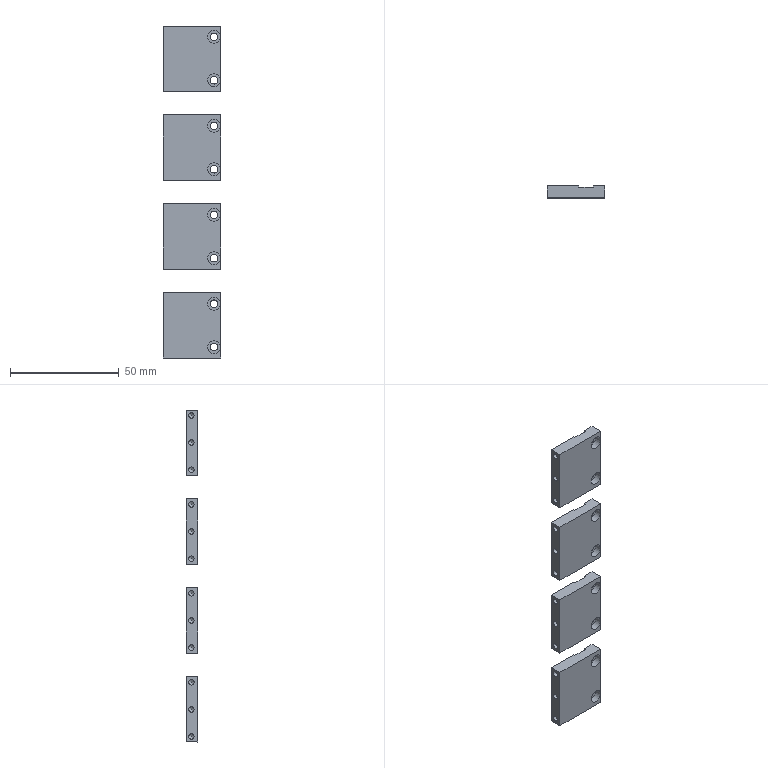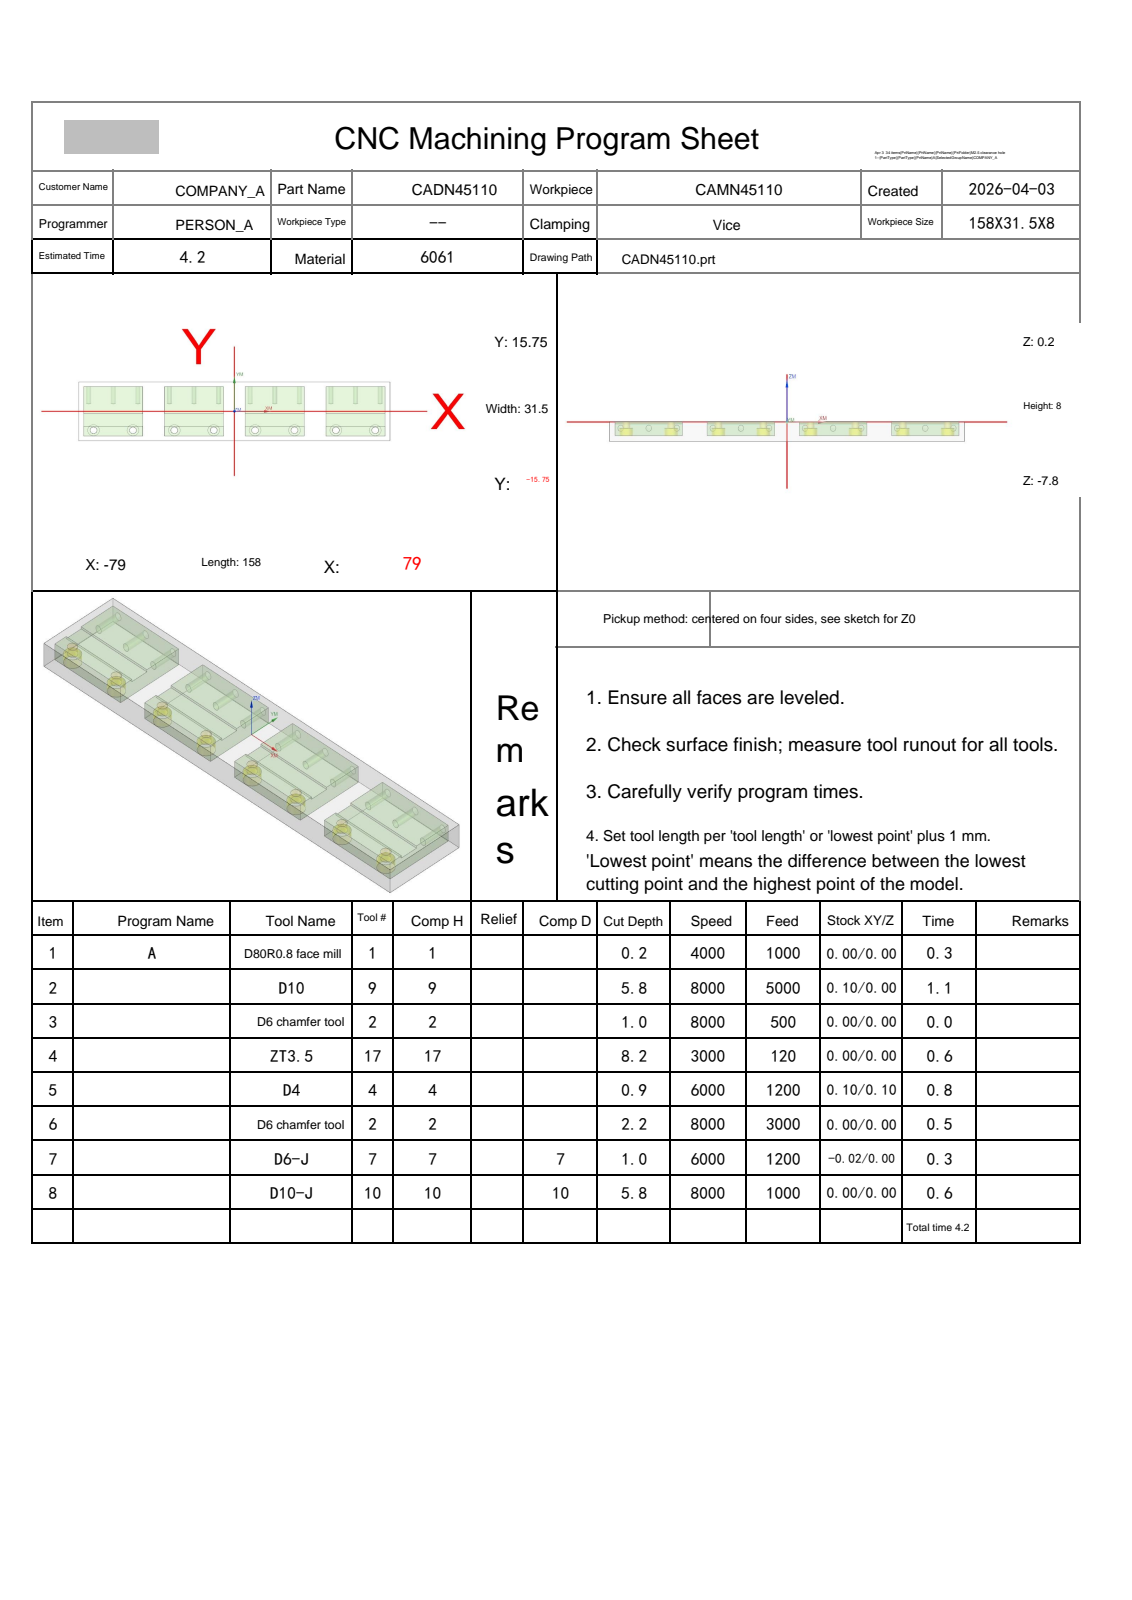NC program | NX | posted by the shop | part box 26.5 x 5.5 x 153 mm
Whole program:
%
O0001
(Machine time: 5.73 MIN)
(===Total Tool:7===)
(T1=D80R0.8 face mill D=80.  R=0.8  D-  H01 Z=-0.   )
(T9=D10     D=10.  R=0.   D-  H09 Z=-5.6  )
(T2=D6 chamfer tool   D=6.   R=0.   D-  H02 Z=-2.05 )
(T17=ZT3.5  D=3.5  DR_a=118 D-  H17 Z=-8.   )
(T4=D4      D=4.   R=0.   D-  H04 Z=-0.66 )
(T7=D6-J    D=6.   R=0.   D7  H07 Z=-0.76 )
(T10=D10-J  D=10.  R=0.   D10 H10 Z=-5.6  )
G80 G90 G17 G49 G40
G91 G28 Z0
M01
N1 T01 M06
(D80R0.8 face mill  D=80. R=0.8 H=01 ce=0.00 di=0.00)
G00 G90 G54 X-121.5 Y0.0 M03 S4000
G43 H01 Z20.
M08
Z2.
G01 Z0.0 F1000.
X-116.5
X116.5
X121.5
Z2.
G00 Z20.
G91 G28 Z0.0
M05
M09
G91 G28 Z0.0
M01
N2 T09 M06
(D10  D=10. R=0. H=09 ce=0.10 di=0.00)
G00 G90 G54 X-61.5 Y18.35 M03 S8000
G43 H09 Z20.
M08
Z.5
G01 X-46.5 Z.421 F5000.
G02 X-41.4 Y13.25 Z.379 I0.0 J-5.1
G01 Y-13.25 Z.24
G02 X-46.5 Y-18.35 Z.198 I-5.1 J0.0
G01 X-76.5 Z.04
G02 X-81.6 Y-13.25 Z-.002 I0.0 J5.1
G01 Y13.25 Z-.142
G02 X-76.5 Y18.35 Z-.184 I5.1 J0.0
G01 X-46.5 Z-.341
G02 X-41.4 Y13.25 Z-.383 I0.0 J-5.1
G01 Y-13.25 Z-.523
G02 X-46.5 Y-18.35 Z-.565 I-5.1 J0.0
G01 X-76.5 Z-.723
G02 X-81.6 Y-13.25 Z-.765 I0.0 J5.1
G01 Y13.25 Z-.904
G02 X-76.5 Y18.35 Z-.946 I5.1 J0.0
G01 X-46.5 Z-1.104
G02 X-41.4 Y13.25 Z-1.146 I0.0 J-5.1
G01 Y-13.25 Z-1.285
G02 X-46.5 Y-18.35 Z-1.327 I-5.1 J0.0
G01 X-76.5 Z-1.485
G02 X-81.6 Y-13.25 Z-1.527 I0.0 J5.1
G01 Y13.25 Z-1.667
G02 X-76.5 Y18.35 Z-1.709 I5.1 J0.0
G01 X-46.5 Z-1.866
G02 X-41.4 Y13.25 Z-1.908 I0.0 J-5.1
G01 Y-13.25 Z-2.048
G02 X-46.5 Y-18.35 Z-2.09 I-5.1 J0.0
G01 X-76.5 Z-2.248
G02 X-81.6 Y-13.25 Z-2.29 I0.0 J5.1
G01 Y13.25 Z-2.429
G02 X-76.5 Y18.35 Z-2.471 I5.1 J0.0
G01 X-46.5 Z-2.629
G02 X-41.4 Y13.25 Z-2.671 I0.0 J-5.1
G01 Y-13.25 Z-2.81
G02 X-46.5 Y-18.35 Z-2.852 I-5.1 J0.0
G01 X-76.5 Z-3.01
G02 X-81.6 Y-13.25 Z-3.052 I0.0 J5.1
G01 Y13.25 Z-3.192
G02 X-76.5 Y18.35 Z-3.234 I5.1 J0.0
G01 X-46.5 Z-3.391
G02 X-41.4 Y13.25 Z-3.433 I0.0 J-5.1
G01 Y-13.25 Z-3.573
G02 X-46.5 Y-18.35 Z-3.615 I-5.1 J0.0
G01 X-76.5 Z-3.773
G02 X-81.6 Y-13.25 Z-3.815 I0.0 J5.1
G01 Y13.25 Z-3.954
G02 X-76.5 Y18.35 Z-3.996 I5.1 J0.0
G01 X-46.5 Z-4.154
G02 X-41.4 Y13.25 Z-4.196 I0.0 J-5.1
G01 Y-13.25 Z-4.335
G02 X-46.5 Y-18.35 Z-4.377 I-5.1 J0.0
G01 X-76.5 Z-4.535
G02 X-81.6 Y-13.25 Z-4.577 I0.0 J5.1
G01 Y13.25 Z-4.717
G02 X-76.5 Y18.35 Z-4.759 I5.1 J0.0
G01 X-46.5 Z-4.916
G02 X-41.4 Y13.25 Z-4.958 I0.0 J-5.1
G01 Y-13.25 Z-5.098
G02 X-46.5 Y-18.35 Z-5.14 I-5.1 J0.0
G01 X-76.5 Z-5.298
G02 X-81.6 Y-13.25 Z-5.34 I0.0 J5.1
G01 Y13.25 Z-5.479
G02 X-76.5 Y18.35 Z-5.521 I5.1 J0.0
G01 X-61.5 Z-5.6
X-46.5
G02 X-41.4 Y13.25 I0.0 J-5.1
G01 Y-13.25
G02 X-46.5 Y-18.35 I-5.1 J0.0
G01 X-76.5
G02 X-81.6 Y-13.25 I0.0 J5.1
G01 Y13.25
G02 X-76.5 Y18.35 I5.1 J0.0
G01 X-61.5
X-61.
Z-4.6
G00 Z20.
X-20.5
Z.5
G01 X-5.5 Z.421
G02 X-.4 Y13.25 Z.379 I0.0 J-5.1
G01 Y-13.25 Z.24
G02 X-5.5 Y-18.35 Z.198 I-5.1 J0.0
G01 X-35.5 Z.04
G02 X-40.6 Y-13.25 Z-.002 I0.0 J5.1
G01 Y13.25 Z-.142
G02 X-35.5 Y18.35 Z-.184 I5.1 J0.0
G01 X-5.5 Z-.341
G02 X-.4 Y13.25 Z-.383 I0.0 J-5.1
G01 Y-13.25 Z-.523
G02 X-5.5 Y-18.35 Z-.565 I-5.1 J0.0
G01 X-35.5 Z-.723
G02 X-40.6 Y-13.25 Z-.765 I0.0 J5.1
G01 Y13.25 Z-.904
G02 X-35.5 Y18.35 Z-.946 I5.1 J0.0
G01 X-5.5 Z-1.104
G02 X-.4 Y13.25 Z-1.146 I0.0 J-5.1
G01 Y-13.25 Z-1.285
G02 X-5.5 Y-18.35 Z-1.327 I-5.1 J0.0
G01 X-35.5 Z-1.485
G02 X-40.6 Y-13.25 Z-1.527 I0.0 J5.1
G01 Y13.25 Z-1.667
G02 X-35.5 Y18.35 Z-1.709 I5.1 J0.0
G01 X-5.5 Z-1.866
G02 X-.4 Y13.25 Z-1.908 I0.0 J-5.1
G01 Y-13.25 Z-2.048
G02 X-5.5 Y-18.35 Z-2.09 I-5.1 J0.0
G01 X-35.5 Z-2.248
G02 X-40.6 Y-13.25 Z-2.29 I0.0 J5.1
G01 Y13.25 Z-2.429
G02 X-35.5 Y18.35 Z-2.471 I5.1 J0.0
G01 X-5.5 Z-2.629
G02 X-.4 Y13.25 Z-2.671 I0.0 J-5.1
G01 Y-13.25 Z-2.81
G02 X-5.5 Y-18.35 Z-2.852 I-5.1 J0.0
G01 X-35.5 Z-3.01
G02 X-40.6 Y-13.25 Z-3.052 I0.0 J5.1
G01 Y13.25 Z-3.192
G02 X-35.5 Y18.35 Z-3.234 I5.1 J0.0
G01 X-5.5 Z-3.391
G02 X-.4 Y13.25 Z-3.433 I0.0 J-5.1
G01 Y-13.25 Z-3.573
G02 X-5.5 Y-18.35 Z-3.615 I-5.1 J0.0
G01 X-35.5 Z-3.773
G02 X-40.6 Y-13.25 Z-3.815 I0.0 J5.1
G01 Y13.25 Z-3.954
G02 X-35.5 Y18.35 Z-3.996 I5.1 J0.0
G01 X-5.5 Z-4.154
G02 X-.4 Y13.25 Z-4.196 I0.0 J-5.1
G01 Y-13.25 Z-4.335
G02 X-5.5 Y-18.35 Z-4.377 I-5.1 J0.0
G01 X-35.5 Z-4.535
G02 X-40.6 Y-13.25 Z-4.577 I0.0 J5.1
G01 Y13.25 Z-4.717
G02 X-35.5 Y18.35 Z-4.759 I5.1 J0.0
G01 X-5.5 Z-4.916
G02 X-.4 Y13.25 Z-4.958 I0.0 J-5.1
G01 Y-13.25 Z-5.098
G02 X-5.5 Y-18.35 Z-5.14 I-5.1 J0.0
G01 X-35.5 Z-5.298
G02 X-40.6 Y-13.25 Z-5.34 I0.0 J5.1
G01 Y13.25 Z-5.479
G02 X-35.5 Y18.35 Z-5.521 I5.1 J0.0
G01 X-20.5 Z-5.6
X-5.5
G02 X-.4 Y13.25 I0.0 J-5.1
G01 Y-13.25
G02 X-5.5 Y-18.35 I-5.1 J0.0
G01 X-35.5
G02 X-40.6 Y-13.25 I0.0 J5.1
G01 Y13.25
G02 X-35.5 Y18.35 I5.1 J0.0
G01 X-20.5
X-20.
Z-4.6
G00 Z20.
X20.5
Z.5
G01 X35.5 Z.421
G02 X40.6 Y13.25 Z.379 I0.0 J-5.1
G01 Y-13.25 Z.24
G02 X35.5 Y-18.35 Z.198 I-5.1 J0.0
G01 X5.5 Z.04
G02 X.4 Y-13.25 Z-.002 I0.0 J5.1
G01 Y13.25 Z-.142
G02 X5.5 Y18.35 Z-.184 I5.1 J0.0
G01 X35.5 Z-.341
G02 X40.6 Y13.25 Z-.383 I0.0 J-5.1
G01 Y-13.25 Z-.523
G02 X35.5 Y-18.35 Z-.565 I-5.1 J0.0
G01 X5.5 Z-.723
G02 X.4 Y-13.25 Z-.765 I0.0 J5.1
G01 Y13.25 Z-.904
G02 X5.5 Y18.35 Z-.946 I5.1 J0.0
G01 X35.5 Z-1.104
G02 X40.6 Y13.25 Z-1.146 I0.0 J-5.1
G01 Y-13.25 Z-1.285
G02 X35.5 Y-18.35 Z-1.327 I-5.1 J0.0
G01 X5.5 Z-1.485
G02 X.4 Y-13.25 Z-1.527 I0.0 J5.1
G01 Y13.25 Z-1.667
G02 X5.5 Y18.35 Z-1.709 I5.1 J0.0
G01 X35.5 Z-1.866
G02 X40.6 Y13.25 Z-1.908 I0.0 J-5.1
G01 Y-13.25 Z-2.048
G02 X35.5 Y-18.35 Z-2.09 I-5.1 J0.0
G01 X5.5 Z-2.248
G02 X.4 Y-13.25 Z-2.29 I0.0 J5.1
G01 Y13.25 Z-2.429
G02 X5.5 Y18.35 Z-2.471 I5.1 J0.0
G01 X35.5 Z-2.629
G02 X40.6 Y13.25 Z-2.671 I0.0 J-5.1
G01 Y-13.25 Z-2.81
G02 X35.5 Y-18.35 Z-2.852 I-5.1 J0.0
G01 X5.5 Z-3.01
G02 X.4 Y-13.25 Z-3.052 I0.0 J5.1
G01 Y13.25 Z-3.192
G02 X5.5 Y18.35 Z-3.234 I5.1 J0.0
G01 X35.5 Z-3.391
G02 X40.6 Y13.25 Z-3.433 I0.0 J-5.1
G01 Y-13.25 Z-3.573
G02 X35.5 Y-18.35 Z-3.615 I-5.1 J0.0
G01 X5.5 Z-3.773
G02 X.4 Y-13.25 Z-3.815 I0.0 J5.1
G01 Y13.25 Z-3.954
G02 X5.5 Y18.35 Z-3.996 I5.1 J0.0
G01 X35.5 Z-4.154
G02 X40.6 Y13.25 Z-4.196 I0.0 J-5.1
G01 Y-13.25 Z-4.335
G02 X35.5 Y-18.35 Z-4.377 I-5.1 J0.0
G01 X5.5 Z-4.535
G02 X.4 Y-13.25 Z-4.577 I0.0 J5.1
G01 Y13.25 Z-4.717
G02 X5.5 Y18.35 Z-4.759 I5.1 J0.0
G01 X35.5 Z-4.916
G02 X40.6 Y13.25 Z-4.958 I0.0 J-5.1
G01 Y-13.25 Z-5.098
G02 X35.5 Y-18.35 Z-5.14 I-5.1 J0.0
G01 X5.5 Z-5.298
G02 X.4 Y-13.25 Z-5.34 I0.0 J5.1
G01 Y13.25 Z-5.479
G02 X5.5 Y18.35 Z-5.521 I5.1 J0.0
G01 X20.5 Z-5.6
X35.5
G02 X40.6 Y13.25 I0.0 J-5.1
G01 Y-13.25
G02 X35.5 Y-18.35 I-5.1 J0.0
G01 X5.5
G02 X.4 Y-13.25 I0.0 J5.1
G01 Y13.25
G02 X5.5 Y18.35 I5.1 J0.0
G01 X20.5
X21.
Z-4.6
G00 Z20.
X61.5
Z.5
G01 X76.5 Z.421
G02 X81.6 Y13.25 Z.379 I0.0 J-5.1
G01 Y-13.25 Z.24
G02 X76.5 Y-18.35 Z.198 I-5.1 J0.0
G01 X46.5 Z.04
G02 X41.4 Y-13.25 Z-.002 I0.0 J5.1
G01 Y13.25 Z-.142
G02 X46.5 Y18.35 Z-.184 I5.1 J0.0
G01 X76.5 Z-.341
G02 X81.6 Y13.25 Z-.383 I0.0 J-5.1
G01 Y-13.25 Z-.523
G02 X76.5 Y-18.35 Z-.565 I-5.1 J0.0
G01 X46.5 Z-.723
G02 X41.4 Y-13.25 Z-.765 I0.0 J5.1
G01 Y13.25 Z-.904
G02 X46.5 Y18.35 Z-.946 I5.1 J0.0
G01 X76.5 Z-1.104
G02 X81.6 Y13.25 Z-1.146 I0.0 J-5.1
G01 Y-13.25 Z-1.285
G02 X76.5 Y-18.35 Z-1.327 I-5.1 J0.0
G01 X46.5 Z-1.485
G02 X41.4 Y-13.25 Z-1.527 I0.0 J5.1
G01 Y13.25 Z-1.667
G02 X46.5 Y18.35 Z-1.709 I5.1 J0.0
G01 X76.5 Z-1.866
G02 X81.6 Y13.25 Z-1.908 I0.0 J-5.1
G01 Y-13.25 Z-2.048
G02 X76.5 Y-18.35 Z-2.09 I-5.1 J0.0
G01 X46.5 Z-2.248
G02 X41.4 Y-13.25 Z-2.29 I0.0 J5.1
G01 Y13.25 Z-2.429
G02 X46.5 Y18.35 Z-2.471 I5.1 J0.0
G01 X76.5 Z-2.629
G02 X81.6 Y13.25 Z-2.671 I0.0 J-5.1
G01 Y-13.25 Z-2.81
G02 X76.5 Y-18.35 Z-2.852 I-5.1 J0.0
G01 X46.5 Z-3.01
G02 X41.4 Y-13.25 Z-3.052 I0.0 J5.1
G01 Y13.25 Z-3.192
G02 X46.5 Y18.35 Z-3.234 I5.1 J0.0
G01 X76.5 Z-3.391
G02 X81.6 Y13.25 Z-3.433 I0.0 J-5.1
G01 Y-13.25 Z-3.573
G02 X76.5 Y-18.35 Z-3.615 I-5.1 J0.0
G01 X46.5 Z-3.773
G02 X41.4 Y-13.25 Z-3.815 I0.0 J5.1
G01 Y13.25 Z-3.954
G02 X46.5 Y18.35 Z-3.996 I5.1 J0.0
G01 X76.5 Z-4.154
G02 X81.6 Y13.25 Z-4.196 I0.0 J-5.1
G01 Y-13.25 Z-4.335
G02 X76.5 Y-18.35 Z-4.377 I-5.1 J0.0
G01 X46.5 Z-4.535
G02 X41.4 Y-13.25 Z-4.577 I0.0 J5.1
G01 Y13.25 Z-4.717
G02 X46.5 Y18.35 Z-4.759 I5.1 J0.0
G01 X76.5 Z-4.916
G02 X81.6 Y13.25 Z-4.958 I0.0 J-5.1
G01 Y-13.25 Z-5.098
G02 X76.5 Y-18.35 Z-5.14 I-5.1 J0.0
G01 X46.5 Z-5.298
G02 X41.4 Y-13.25 Z-5.34 I0.0 J5.1
G01 Y13.25 Z-5.479
G02 X46.5 Y18.35 Z-5.521 I5.1 J0.0
G01 X61.5 Z-5.6
X76.5
G02 X81.6 Y13.25 I0.0 J-5.1
G01 Y-13.25
G02 X76.5 Y-18.35 I-5.1 J0.0
G01 X46.5
G02 X41.4 Y-13.25 I0.0 J5.1
G01 Y13.25
G02 X46.5 Y18.35 I5.1 J0.0
G01 X61.5
X62.
Z-4.6
G00 Z20.
G91 G28 Z0.0
M05
M09
G91 G28 Z0.0
M01
N3 T02 M06
(D6 chamfer tool  D=6. R=0. H=02 ce=0.00 di=0.00)
G00 G90 G54 X-71.5 Y-10.15 M03 S8000
G43 H02 Z20.
M08
G98 G81 X-71.5 Y-10.15 Z-.8 R1. F500.
X-51.5
X-30.5
X-10.5
X10.5
X30.5
X51.5
X71.5
G80
G00 Z20.
G91 G28 Z0.0
M05
M09
G91 G28 Z0.0
M01
N4 T17 M06
(ZT3.5 D=3.5 DR_a=118 H=17)
G00 G90 G54 X-71.5 Y-10.15 M03 S3000
G43 H17 Z20.
M08
G98 G83 X-71.5 Y-10.15 Z-8. R1. F120. Q3.
X-51.5
X-30.5
X-10.5
X10.5
X30.5
X51.5
X71.5
G80
G00 Z20.
G91 G28 Z0.0
M05
M09
G91 G28 Z0.0
M01
N5 T04 M06
(D4  D=4. R=0. H=04 ce=0.10 di=0.10)
G00 G90 G54 X-81.6 Y-4.65 M03 S6000
G43 H04 Z20.
M08
Z.281
G01 Z-.219 F1200.
X-76.9
Y-5.95
X-46.1
Y-3.35
X-76.9
Y-4.65
Y-5.15
Z.281
G00 Z.5
X-81.6 Y-4.65
Z.062
G01 Z-.438
X-76.9
Y-5.95
X-46.1
Y-3.35
X-76.9
Y-4.65
Y-5.15
Z.062
G00 Z.281
X-81.6 Y-4.65
Z-.157
G01 Z-.657
X-76.9
Y-5.95
X-46.1
Y-3.35
X-76.9
Y-4.65
Y-5.15
Z-.157
G00 Z20.
X-40.6 Y-4.65
Z.281
G01 Z-.219
X-35.9
Y-5.95
X-5.1
Y-3.35
X-35.9
Y-4.65
Y-5.15
Z.281
G00 Z.5
X-40.6 Y-4.65
Z.062
G01 Z-.438
X-35.9
Y-5.95
X-5.1
Y-3.35
X-35.9
Y-4.65
Y-5.15
Z.062
G00 Z.281
X-40.6 Y-4.65
Z-.157
G01 Z-.657
X-35.9
Y-5.95
X-5.1
Y-3.35
X-35.9
Y-4.65
Y-5.15
Z-.157
G00 Z20.
X.4 Y-4.65
Z.281
G01 Z-.219
X5.1
Y-5.95
X35.9
Y-3.35
X5.1
Y-4.65
Y-5.15
Z.281
G00 Z.5
X.4 Y-4.65
Z.062
G01 Z-.438
X5.1
Y-5.95
X35.9
Y-3.35
X5.1
Y-4.65
Y-5.15
Z.062
G00 Z.281
X.4 Y-4.65
Z-.157
G01 Z-.657
X5.1
Y-5.95
X35.9
Y-3.35
X5.1
Y-4.65
Y-5.15
Z-.157
G00 Z20.
X81.6 Y-4.65
Z.281
G01 Z-.219
X76.9
Y-3.35
X46.1
Y-5.95
X76.9
Y-4.65
Y-4.15
Z.281
G00 Z.5
X81.6 Y-4.65
Z.062
G01 Z-.438
X76.9
Y-3.35
X46.1
Y-5.95
X76.9
Y-4.65
Y-4.15
Z.062
G00 Z.281
X81.6 Y-4.65
Z-.157
G01 Z-.657
X76.9
Y-3.35
X46.1
Y-5.95
X76.9
Y-4.65
Y-4.15
Z-.157
G00 Z20.
G91 G28 Z0.0
M05
M09
G91 G28 Z0.0
M01
N6 T02 M06
(D6 chamfer tool  D=6. R=0. H=02 ce=0.00 di=0.00)
G00 G90 G54 X-61.75 Y-6.872 M03 S8000
G43 H02 Z20.
M08
Z2.985
G01 Z-.499 F3000.
G03 X-61.83 Y-7.172 I.52 J-.3
X-61.53 Y-7.692 I.6 J0.0
G01 X-61.5 Y-7.7
X-46.5
X-46.366 Y-7.727
X-46.253 Y-7.803
X-46.177 Y-7.916
X-46.15 Y-8.05
Y-13.25
X-46.177 Y-13.384
X-46.253 Y-13.497
X-46.366 Y-13.573
X-46.5 Y-13.6
X-76.5
X-76.634 Y-13.573
X-76.747 Y-13.497
X-76.823 Y-13.384
X-76.85 Y-13.25
Y-8.05
X-76.823 Y-7.916
X-76.747 Y-7.803
X-76.634 Y-7.727
X-76.5 Y-7.7
X-61.5
X-61.47 Y-7.692
G03 X-61.17 Y-7.172 I-.3 J.52
X-61.25 Y-6.872 I-.6 J0.0
G01 Z2.985
G00 Z3.251
Y-2.428
Z2.985
G01 Z-.499
G03 X-61.17 Y-2.128 I-.52 J.3
X-61.47 Y-1.608 I-.6 J0.0
G01 X-61.5 Y-1.6
X-76.5
X-76.634 Y-1.573
X-76.747 Y-1.497
X-76.823 Y-1.384
X-76.85 Y-1.25
Y13.25
X-76.823 Y13.384
X-76.747 Y13.497
X-76.634 Y13.573
X-76.5 Y13.6
X-46.5
X-46.366 Y13.573
X-46.253 Y13.497
X-46.177 Y13.384
X-46.15 Y13.25
Y-1.25
X-46.177 Y-1.384
X-46.253 Y-1.497
X-46.366 Y-1.573
X-46.5 Y-1.6
X-61.5
X-61.53 Y-1.608
G03 X-61.83 Y-2.128 I.3 J-.52
X-61.75 Y-2.428 I.6 J0.0
G01 Z2.985
G00 Z20.
X-20.25 Y-14.428
Z2.985
G01 Z-.499
G03 X-20.17 Y-14.128 I-.52 J.3
X-20.47 Y-13.608 I-.6 J0.0
G01 X-20.5 Y-13.6
X-35.5
X-35.634 Y-13.573
X-35.747 Y-13.497
X-35.823 Y-13.384
X-35.85 Y-13.25
Y-8.05
X-35.823 Y-7.916
X-35.747 Y-7.803
X-35.634 Y-7.727
X-35.5 Y-7.7
X-5.5
X-5.366 Y-7.727
X-5.253 Y-7.803
X-5.177 Y-7.916
X-5.15 Y-8.05
Y-13.25
X-5.177 Y-13.384
X-5.253 Y-13.497
X-5.366 Y-13.573
X-5.5 Y-13.6
X-20.5
X-20.53 Y-13.608
G03 X-20.83 Y-14.128 I.3 J-.52
X-20.75 Y-14.428 I.6 J0.0
G01 Z2.985
G00 Z20.
X-20.25 Y-2.428
Z2.985
G01 Z-.499
G03 X-20.17 Y-2.128 I-.52 J.3
X-20.47 Y-1.608 I-.6 J0.0
G01 X-20.5 Y-1.6
X-35.5
X-35.634 Y-1.573
X-35.747 Y-1.497
X-35.823 Y-1.384
X-35.85 Y-1.25
Y13.25
X-35.823 Y13.384
X-35.747 Y13.497
X-35.634 Y13.573
X-35.5 Y13.6
X-5.5
X-5.366 Y13.573
X-5.253 Y13.497
X-5.177 Y13.384
X-5.15 Y13.25
Y-1.25
X-5.177 Y-1.384
X-5.253 Y-1.497
X-5.366 Y-1.573
X-5.5 Y-1.6
X-20.5
X-20.53 Y-1.608
G03 X-20.83 Y-2.128 I.3 J-.52
X-20.75 Y-2.428 I.6 J0.0
G01 Z2.985
G00 Z20.
X20.75 Y-14.428
Z2.985
G01 Z-.499
G03 X20.83 Y-14.128 I-.52 J.3
X20.53 Y-13.608 I-.6 J0.0
G01 X20.5 Y-13.6
X5.5
X5.366 Y-13.573
X5.253 Y-13.497
X5.177 Y-13.384
X5.15 Y-13.25
Y-8.05
X5.177 Y-7.916
X5.253 Y-7.803
X5.366 Y-7.727
X5.5 Y-7.7
X35.5
X35.634 Y-7.727
X35.747 Y-7.803
X35.823 Y-7.916
X35.85 Y-8.05
Y-13.25
X35.823 Y-13.384
X35.747 Y-13.497
X35.634 Y-13.573
X35.5 Y-13.6
X20.5
X20.47 Y-13.608
G03 X20.17 Y-14.128 I.3 J-.52
X20.25 Y-14.428 I.6 J0.0
G01 Z2.985
G00 Z20.
X20.75 Y-2.428
Z2.985
G01 Z-.499
G03 X20.83 Y-2.128 I-.52 J.3
X20.53 Y-1.608 I-.6 J0.0
G01 X20.5 Y-1.6
X5.5
X5.366 Y-1.573
X5.253 Y-1.497
X5.177 Y-1.384
X5.15 Y-1.25
Y13.25
X5.177 Y13.384
X5.253 Y13.497
X5.366 Y13.573
X5.5 Y13.6
X35.5
X35.634 Y13.573
X35.747 Y13.497
X35.823 Y13.384
X35.85 Y13.25
Y-1.25
X35.823 Y-1.384
X35.747 Y-1.497
X35.634 Y-1.573
X35.5 Y-1.6
X20.5
X20.47 Y-1.608
G03 X20.17 Y-2.128 I.3 J-.52
X20.25 Y-2.428 I.6 J0.0
G01 Z2.985
G00 Z20.
X61.75 Y-14.428
Z2.985
G01 Z-.499
G03 X61.83 Y-14.128 I-.52 J.3
X61.53 Y-13.608 I-.6 J0.0
G01 X61.5 Y-13.6
X46.5
X46.366 Y-13.573
X46.253 Y-13.497
X46.177 Y-13.384
X46.15 Y-13.25
Y-8.05
X46.177 Y-7.916
X46.253 Y-7.803
X46.366 Y-7.727
X46.5 Y-7.7
X76.5
X76.634 Y-7.727
X76.747 Y-7.803
X76.823 Y-7.916
X76.85 Y-8.05
Y-13.25
X76.823 Y-13.384
X76.747 Y-13.497
X76.634 Y-13.573
X76.5 Y-13.6
X61.5
X61.47 Y-13.608
G03 X61.17 Y-14.128 I.3 J-.52
X61.25 Y-14.428 I.6 J0.0
G01 Z2.985
G00 Z20.
X61.75 Y-2.428
Z2.985
G01 Z-.499
G03 X61.83 Y-2.128 I-.52 J.3
X61.53 Y-1.608 I-.6 J0.0
G01 X61.5 Y-1.6
X46.5
X46.366 Y-1.573
X46.253 Y-1.497
X46.177 Y-1.384
X46.15 Y-1.25
Y13.25
X46.177 Y13.384
X46.253 Y13.497
X46.366 Y13.573
X46.5 Y13.6
X76.5
X76.634 Y13.573
X76.747 Y13.497
X76.823 Y13.384
X76.85 Y13.25
Y-1.25
X76.823 Y-1.384
X76.747 Y-1.497
X76.634 Y-1.573
X76.5 Y-1.6
X61.5
X61.47 Y-1.608
G03 X61.17 Y-2.128 I.3 J-.52
X61.25 Y-2.428 I.6 J0.0
G01 Z2.985
G00 Z20.
X46.15 Y-6.855
Z2.982
G01 Z-1.256
Y-2.445
Z2.982
G00 Z20.
X76.85
Z2.982
G01 Z-1.256
Y-6.855
Z2.982
G00 Z20.
X5.15
Z2.982
G01 Z-1.256
Y-2.445
Z2.982
G00 Z20.
X35.85
Z2.982
G01 Z-1.256
Y-6.855
Z2.982
G00 Z20.
X-35.85
Z2.982
G01 Z-1.256
Y-2.445
Z2.982
G00 Z20.
X-5.15
Z2.982
G01 Z-1.256
Y-6.855
Z2.982
G00 Z20.
X-76.85
Z2.982
G01 Z-1.256
Y-2.445
Z2.982
G00 Z20.
X-46.15
Z2.982
G01 Z-1.256
Y-6.855
Z2.982
G00 Z20.
G00 G90 X-71.5 Y-10.15 M03 S8000
Z20.
G98 G81 X-71.5 Y-10.15 Z-2.05 R3. F500.
X-51.5
X-30.5
X-10.5
X10.5
X30.5
X51.5
X71.5
G80
G00 Z20.
G91 G28 Z0.0
M05
M09
G91 G28 Z0.0
M01
N7 T07 M06
(D6-J  D=6. R=0. H=07 ce=-0.02 di=0.00)
G00 G90 G54 X80.58 Y-5.23 M03 S6000
G43 H07 Z20.
M08
Z-.257
G01 Z-.757 F1200.
G41 D07
X80.2
G03 X79.2 Y-4.23 I-1. J0.0
G01 X43.8
G03 X42.8 Y-5.23 I0.0 J-1.
G01 G40 Y-5.33
Y-3.97
G41 D07
Y-4.07
G03 X43.8 Y-5.07 I1. J0.0
G01 X79.2
G03 X80.2 Y-4.07 I0.0 J1.
G01 X80.48
G40 X80.58
Z-.257
G00 Z20.
X39.58 Y-5.23
Z-.257
G01 Z-.757
G41 D07
X39.2
G03 X38.2 Y-4.23 I-1. J0.0
G01 X2.8
G03 X1.8 Y-5.23 I0.0 J-1.
G01 G40 Y-5.33
Y-3.97
G41 D07
Y-4.07
G03 X2.8 Y-5.07 I1. J0.0
G01 X38.2
G03 X39.2 Y-4.07 I0.0 J1.
G01 X39.48
G40 X39.58
Z-.257
G00 Z20.
X-1.42 Y-5.23
Z-.257
G01 Z-.757
G41 D07
X-1.8
G03 X-2.8 Y-4.23 I-1. J0.0
G01 X-38.2
G03 X-39.2 Y-5.23 I0.0 J-1.
G01 G40 Y-5.33
Y-3.97
G41 D07
Y-4.07
G03 X-38.2 Y-5.07 I1. J0.0
G01 X-2.8
G03 X-1.8 Y-4.07 I0.0 J1.
G01 X-1.52
G40 X-1.42
Z-.257
G00 Z20.
X-42.42 Y-5.23
Z-.257
G01 Z-.757
G41 D07
X-42.8
G03 X-43.8 Y-4.23 I-1. J0.0
G01 X-79.2
G03 X-80.2 Y-5.23 I0.0 J-1.
G01 G40 Y-5.33
Y-3.97
G41 D07
Y-4.07
G03 X-79.2 Y-5.07 I1. J0.0
G01 X-43.8
G03 X-42.8 Y-4.07 I0.0 J1.
G01 X-42.52
G40 X-42.42
Z-.257
G00 Z20.
G91 G28 Z0.0
M05
M09
G91 G28 Z0.0
M01
N8 T10 M06
(D10-J  D=10. R=0. H=10 ce=0.00 di=0.00)
G00 G90 G54 X-77.513 Y19.366 M03 S8000
G43 H10 Z20.
M08
Z-5.1
G01 Z-5.6 F1000.
G41 D10
X-77.497 Y19.167
G03 X-76.5 Y18.25 I.997 J.083
G01 X-46.5
G02 X-41.5 Y13.25 I0.0 J-5.
G01 Y-13.25
G02 X-46.5 Y-18.25 I-5. J0.0
G01 X-76.5
G02 X-81.5 Y-13.25 I0.0 J5.
G01 Y13.25
G02 X-76.5 Y18.25 I5. J0.0
G01 X-76.
G03 X-75. Y19.25 I0.0 J1.
G01 G40 Y19.45
Z-5.1
G00 Z20.
X-21.5
Z-5.1
G01 Z-5.6
G41 D10
Y19.25
G03 X-20.5 Y18.25 I1. J0.0
G01 X-5.5
G02 X-.5 Y13.25 I0.0 J-5.
G01 Y-13.25
G02 X-5.5 Y-18.25 I-5. J0.0
G01 X-35.5
G02 X-40.5 Y-13.25 I0.0 J5.
G01 Y13.25
G02 X-35.5 Y18.25 I5. J0.0
G01 X-20.5
X-20.
G03 X-19. Y19.25 I0.0 J1.
G01 G40 Y19.45
Z-5.1
G00 Z20.
X19.5
Z-5.1
G01 Z-5.6
G41 D10
Y19.25
G03 X20.5 Y18.25 I1. J0.0
G01 X35.5
G02 X40.5 Y13.25 I0.0 J-5.
G01 Y-13.25
G02 X35.5 Y-18.25 I-5. J0.0
G01 X5.5
G02 X.5 Y-13.25 I0.0 J5.
G01 Y13.25
G02 X5.5 Y18.25 I5. J0.0
G01 X20.5
X21.
G03 X22. Y19.25 I0.0 J1.
G01 G40 Y19.45
Z-5.1
G00 Z20.
X60.5
Z-5.1
G01 Z-5.6
G41 D10
Y19.25
G03 X61.5 Y18.25 I1. J0.0
G01 X76.5
G02 X81.5 Y13.25 I0.0 J-5.
G01 Y-13.25
G02 X76.5 Y-18.25 I-5. J0.0
G01 X46.5
G02 X41.5 Y-13.25 I0.0 J5.
G01 Y13.25
G02 X46.5 Y18.25 I5. J0.0
G01 X61.5
X62.
G03 X63. Y19.25 I0.0 J1.
G01 G40 Y19.45
Z-5.1
G00 Z20.
M05
M09
G91 G28 Z0.0
G91 G28 Y0.0
M30
%